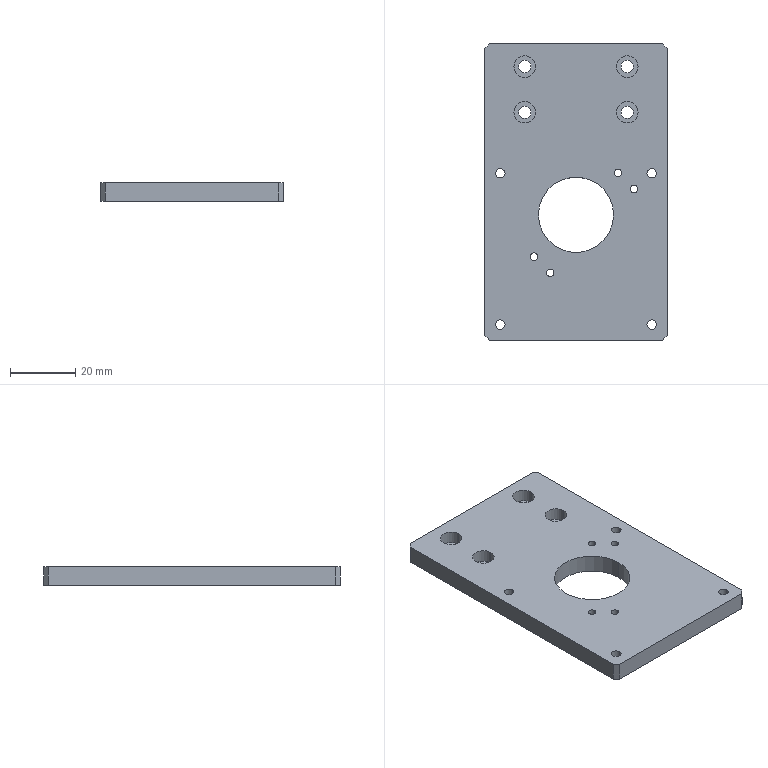Part | SolidWorks | features SplitBody 1 | 1 solid | 48 faces | box 56 x 91 x 5.6 mm | volume 25293 mm3 | cylinder 34 | plane 14 | commonest cylinder face diameters 2.31 x8 2.94 x8 3.85 x8 6.65 x8 23.1 x2